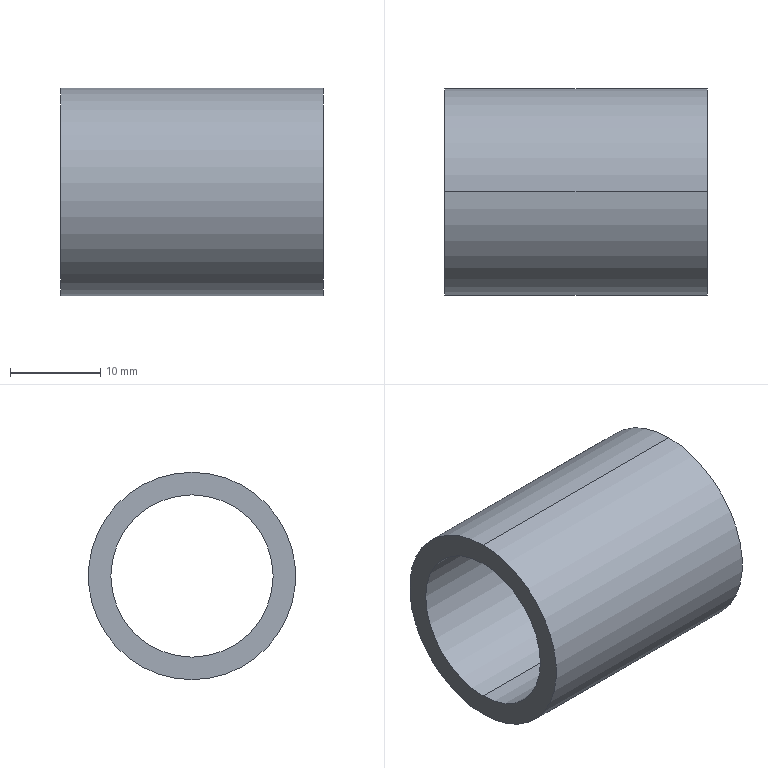Part | STEP file | Completa.sldasm-Part-1_Valor predeterminado | 1 solid | 6 faces | box 29.178 x 23 x 23 mm | volume 4698 mm3 | cylinder 4 | plane 2 | commonest cylinder face diameters 18 x2 23 x2
STEP:
#1=CARTESIAN_POINT('',(0.,0.,0.));
#2=DIRECTION('',(0.,0.,1.));
#3=DIRECTION('',(1.,0.,0.));
#4=AXIS2_PLACEMENT_3D('',#1,#2,#3);
#5=CARTESIAN_POINT('',(-311.426,0.,9.));
#6=VERTEX_POINT('',#5);
#7=CARTESIAN_POINT('',(-340.603,0.,9.));
#8=VERTEX_POINT('',#7);
#9=CARTESIAN_POINT('',(-317.916,0.,9.));
#10=DIRECTION('',(-1.,0.,0.));
#11=VECTOR('',#10,1.);
#12=LINE('',#9,#11);
#13=CARTESIAN_POINT('',(-317.916,0.,0.));
#14=DIRECTION('',(-1.,0.,0.));
#15=DIRECTION('',(0.,0.,1.));
#16=AXIS2_PLACEMENT_3D('',#13,#14,#15);
#17=CYLINDRICAL_SURFACE('',#16,9.);
#18=CARTESIAN_POINT('',(6.283,0.));
#19=DIRECTION('',(0.,1.));
#20=VECTOR('',#19,1.);
#21=LINE('',#18,#20);
#22=(GEOMETRIC_REPRESENTATION_CONTEXT(2)PARAMETRIC_REPRESENTATION_CONTEXT()REPRESENTATION_CONTEXT('',''));
#23=DEFINITIONAL_REPRESENTATION('',(#21),#22);
#24=PCURVE('',#17,#23);
#25=CARTESIAN_POINT('',(-317.916,0.,0.));
#26=DIRECTION('',(-1.,0.,0.));
#27=DIRECTION('',(0.,0.,1.));
#28=AXIS2_PLACEMENT_3D('',#25,#26,#27);
#29=CYLINDRICAL_SURFACE('',#28,9.);
#30=CARTESIAN_POINT('',(0.,0.));
#31=DIRECTION('',(0.,1.));
#32=VECTOR('',#31,1.);
#33=LINE('',#30,#32);
#34=(GEOMETRIC_REPRESENTATION_CONTEXT(2)PARAMETRIC_REPRESENTATION_CONTEXT()REPRESENTATION_CONTEXT('',''));
#35=DEFINITIONAL_REPRESENTATION('',(#33),#34);
#36=PCURVE('',#29,#35);
#37=SURFACE_CURVE('',#12,(#24,#36),.PCURVE_S1.);
#38=EDGE_CURVE('',#6,#8,#37,.T.);
#39=ORIENTED_EDGE('',*,*,#38,.T.);
#40=CARTESIAN_POINT('',(-340.603,0.,-9.));
#41=VERTEX_POINT('',#40);
#42=CARTESIAN_POINT('',(-340.603,0.,0.));
#43=DIRECTION('',(-1.,0.,0.));
#44=DIRECTION('',(0.,0.,-1.));
#45=AXIS2_PLACEMENT_3D('',#42,#43,#44);
#46=CIRCLE('',#45,9.);
#47=CARTESIAN_POINT('',(3.142,22.687));
#48=DIRECTION('',(1.,0.));
#49=VECTOR('',#48,1.);
#50=LINE('',#47,#49);
#51=(GEOMETRIC_REPRESENTATION_CONTEXT(2)PARAMETRIC_REPRESENTATION_CONTEXT()REPRESENTATION_CONTEXT('',''));
#52=DEFINITIONAL_REPRESENTATION('',(#50),#51);
#53=PCURVE('',#17,#52);
#54=CARTESIAN_POINT('',(-340.603,0.,0.));
#55=DIRECTION('',(1.,0.,0.));
#56=DIRECTION('',(0.,0.,-1.));
#57=AXIS2_PLACEMENT_3D('',#54,#55,#56);
#58=PLANE('',#57);
#59=CARTESIAN_POINT('',(9.,0.));
#60=CARTESIAN_POINT('',(9.,-15.588));
#61=CARTESIAN_POINT('',(-4.5,-7.794));
#62=CARTESIAN_POINT('',(-18.,0.));
#63=CARTESIAN_POINT('',(-4.5,7.794));
#64=CARTESIAN_POINT('',(9.,15.588));
#65=CARTESIAN_POINT('',(9.,0.));
#66=(BOUNDED_CURVE()B_SPLINE_CURVE(2,(#59,#60,#61,#62,#63,#64,#65),.UNSPECIFIED.,.T.,.F.)B_SPLINE_CURVE_WITH_KNOTS((1,2,2,2,2,1),(-2.094,0.,2.094,4.189,6.283,8.378),.UNSPECIFIED.)CURVE()GEOMETRIC_REPRESENTATION_ITEM()RATIONAL_B_SPLINE_CURVE((1.,0.5,1.,0.5,1.,0.5,1.))REPRESENTATION_ITEM(''));
#67=(GEOMETRIC_REPRESENTATION_CONTEXT(2)PARAMETRIC_REPRESENTATION_CONTEXT()REPRESENTATION_CONTEXT('',''));
#68=DEFINITIONAL_REPRESENTATION('',(#66),#67);
#69=PCURVE('',#58,#68);
#70=SURFACE_CURVE('',#46,(#53,#69),.PCURVE_S1.);
#71=EDGE_CURVE('',#41,#8,#70,.T.);
#72=ORIENTED_EDGE('',*,*,#71,.F.);
#73=CARTESIAN_POINT('',(-311.426,0.,-9.));
#74=VERTEX_POINT('',#73);
#75=CARTESIAN_POINT('',(-317.916,0.,-9.));
#76=DIRECTION('',(-1.,0.,0.));
#77=VECTOR('',#76,1.);
#78=LINE('',#75,#77);
#79=CARTESIAN_POINT('',(3.142,0.));
#80=DIRECTION('',(0.,1.));
#81=VECTOR('',#80,1.);
#82=LINE('',#79,#81);
#83=(GEOMETRIC_REPRESENTATION_CONTEXT(2)PARAMETRIC_REPRESENTATION_CONTEXT()REPRESENTATION_CONTEXT('',''));
#84=DEFINITIONAL_REPRESENTATION('',(#82),#83);
#85=PCURVE('',#17,#84);
#86=CARTESIAN_POINT('',(3.142,0.));
#87=DIRECTION('',(0.,1.));
#88=VECTOR('',#87,1.);
#89=LINE('',#86,#88);
#90=(GEOMETRIC_REPRESENTATION_CONTEXT(2)PARAMETRIC_REPRESENTATION_CONTEXT()REPRESENTATION_CONTEXT('',''));
#91=DEFINITIONAL_REPRESENTATION('',(#89),#90);
#92=PCURVE('',#29,#91);
#93=SURFACE_CURVE('',#78,(#85,#92),.PCURVE_S1.);
#94=EDGE_CURVE('',#74,#41,#93,.T.);
#95=ORIENTED_EDGE('',*,*,#94,.F.);
#96=CARTESIAN_POINT('',(-311.426,0.,0.));
#97=DIRECTION('',(1.,0.,0.));
#98=DIRECTION('',(0.,0.,1.));
#99=AXIS2_PLACEMENT_3D('',#96,#97,#98);
#100=CIRCLE('',#99,9.);
#101=CARTESIAN_POINT('',(6.283,-6.49));
#102=DIRECTION('',(-1.,0.));
#103=VECTOR('',#102,1.);
#104=LINE('',#101,#103);
#105=(GEOMETRIC_REPRESENTATION_CONTEXT(2)PARAMETRIC_REPRESENTATION_CONTEXT()REPRESENTATION_CONTEXT('',''));
#106=DEFINITIONAL_REPRESENTATION('',(#104),#105);
#107=PCURVE('',#17,#106);
#108=CARTESIAN_POINT('',(-311.426,0.,0.));
#109=DIRECTION('',(-1.,0.,0.));
#110=DIRECTION('',(0.,0.,1.));
#111=AXIS2_PLACEMENT_3D('',#108,#109,#110);
#112=PLANE('',#111);
#113=CARTESIAN_POINT('',(9.,0.));
#114=CARTESIAN_POINT('',(9.,-15.588));
#115=CARTESIAN_POINT('',(-4.5,-7.794));
#116=CARTESIAN_POINT('',(-18.,0.));
#117=CARTESIAN_POINT('',(-4.5,7.794));
#118=CARTESIAN_POINT('',(9.,15.588));
#119=CARTESIAN_POINT('',(9.,0.));
#120=(BOUNDED_CURVE()B_SPLINE_CURVE(2,(#113,#114,#115,#116,#117,#118,#119),.UNSPECIFIED.,.T.,.F.)B_SPLINE_CURVE_WITH_KNOTS((1,2,2,2,2,1),(-2.094,0.,2.094,4.189,6.283,8.378),.UNSPECIFIED.)CURVE()GEOMETRIC_REPRESENTATION_ITEM()RATIONAL_B_SPLINE_CURVE((1.,0.5,1.,0.5,1.,0.5,1.))REPRESENTATION_ITEM(''));
#121=(GEOMETRIC_REPRESENTATION_CONTEXT(2)PARAMETRIC_REPRESENTATION_CONTEXT()REPRESENTATION_CONTEXT('',''));
#122=DEFINITIONAL_REPRESENTATION('',(#120),#121);
#123=PCURVE('',#112,#122);
#124=SURFACE_CURVE('',#100,(#107,#123),.PCURVE_S1.);
#125=EDGE_CURVE('',#6,#74,#124,.T.);
#126=ORIENTED_EDGE('',*,*,#125,.F.);
#127=EDGE_LOOP('',(#39,#72,#95,#126));
#128=FACE_BOUND('',#127,.F.);
#129=ADVANCED_FACE('',(#128),#17,.F.);
#130=CARTESIAN_POINT('',(-311.426,0.,-11.5));
#131=VERTEX_POINT('',#130);
#132=CARTESIAN_POINT('',(-311.426,0.,11.5));
#133=VERTEX_POINT('',#132);
#134=CARTESIAN_POINT('',(-311.426,0.,0.));
#135=DIRECTION('',(1.,0.,0.));
#136=DIRECTION('',(0.,0.,1.));
#137=AXIS2_PLACEMENT_3D('',#134,#135,#136);
#138=CIRCLE('',#137,11.5);
#139=CARTESIAN_POINT('',(-317.916,0.,0.));
#140=DIRECTION('',(-1.,0.,0.));
#141=DIRECTION('',(0.,0.,1.));
#142=AXIS2_PLACEMENT_3D('',#139,#140,#141);
#143=CYLINDRICAL_SURFACE('',#142,11.5);
#144=CARTESIAN_POINT('',(6.283,-6.49));
#145=DIRECTION('',(-1.,0.));
#146=VECTOR('',#145,1.);
#147=LINE('',#144,#146);
#148=(GEOMETRIC_REPRESENTATION_CONTEXT(2)PARAMETRIC_REPRESENTATION_CONTEXT()REPRESENTATION_CONTEXT('',''));
#149=DEFINITIONAL_REPRESENTATION('',(#147),#148);
#150=PCURVE('',#143,#149);
#151=CARTESIAN_POINT('',(11.5,0.));
#152=CARTESIAN_POINT('',(11.5,-19.919));
#153=CARTESIAN_POINT('',(-5.75,-9.959));
#154=CARTESIAN_POINT('',(-23.,0.));
#155=CARTESIAN_POINT('',(-5.75,9.959));
#156=CARTESIAN_POINT('',(11.5,19.919));
#157=CARTESIAN_POINT('',(11.5,0.));
#158=(BOUNDED_CURVE()B_SPLINE_CURVE(2,(#151,#152,#153,#154,#155,#156,#157),.UNSPECIFIED.,.T.,.F.)B_SPLINE_CURVE_WITH_KNOTS((1,2,2,2,2,1),(-2.094,0.,2.094,4.189,6.283,8.378),.UNSPECIFIED.)CURVE()GEOMETRIC_REPRESENTATION_ITEM()RATIONAL_B_SPLINE_CURVE((1.,0.5,1.,0.5,1.,0.5,1.))REPRESENTATION_ITEM(''));
#159=(GEOMETRIC_REPRESENTATION_CONTEXT(2)PARAMETRIC_REPRESENTATION_CONTEXT()REPRESENTATION_CONTEXT('',''));
#160=DEFINITIONAL_REPRESENTATION('',(#158),#159);
#161=PCURVE('',#112,#160);
#162=SURFACE_CURVE('',#138,(#150,#161),.PCURVE_S1.);
#163=EDGE_CURVE('',#131,#133,#162,.T.);
#164=ORIENTED_EDGE('',*,*,#163,.F.);
#165=CARTESIAN_POINT('',(-340.603,0.,-11.5));
#166=VERTEX_POINT('',#165);
#167=CARTESIAN_POINT('',(-317.916,0.,-11.5));
#168=DIRECTION('',(-1.,0.,0.));
#169=VECTOR('',#168,1.);
#170=LINE('',#167,#169);
#171=CARTESIAN_POINT('',(3.142,0.));
#172=DIRECTION('',(0.,1.));
#173=VECTOR('',#172,1.);
#174=LINE('',#171,#173);
#175=(GEOMETRIC_REPRESENTATION_CONTEXT(2)PARAMETRIC_REPRESENTATION_CONTEXT()REPRESENTATION_CONTEXT('',''));
#176=DEFINITIONAL_REPRESENTATION('',(#174),#175);
#177=PCURVE('',#143,#176);
#178=CARTESIAN_POINT('',(-317.916,0.,0.));
#179=DIRECTION('',(-1.,0.,0.));
#180=DIRECTION('',(0.,0.,1.));
#181=AXIS2_PLACEMENT_3D('',#178,#179,#180);
#182=CYLINDRICAL_SURFACE('',#181,11.5);
#183=CARTESIAN_POINT('',(3.142,0.));
#184=DIRECTION('',(0.,1.));
#185=VECTOR('',#184,1.);
#186=LINE('',#183,#185);
#187=(GEOMETRIC_REPRESENTATION_CONTEXT(2)PARAMETRIC_REPRESENTATION_CONTEXT()REPRESENTATION_CONTEXT('',''));
#188=DEFINITIONAL_REPRESENTATION('',(#186),#187);
#189=PCURVE('',#182,#188);
#190=SURFACE_CURVE('',#170,(#177,#189),.PCURVE_S1.);
#191=EDGE_CURVE('',#131,#166,#190,.T.);
#192=ORIENTED_EDGE('',*,*,#191,.T.);
#193=CARTESIAN_POINT('',(-340.603,0.,11.5));
#194=VERTEX_POINT('',#193);
#195=CARTESIAN_POINT('',(-340.603,0.,0.));
#196=DIRECTION('',(-1.,0.,0.));
#197=DIRECTION('',(0.,0.,-1.));
#198=AXIS2_PLACEMENT_3D('',#195,#196,#197);
#199=CIRCLE('',#198,11.5);
#200=CARTESIAN_POINT('',(-3.142,22.687));
#201=DIRECTION('',(1.,0.));
#202=VECTOR('',#201,1.);
#203=LINE('',#200,#202);
#204=(GEOMETRIC_REPRESENTATION_CONTEXT(2)PARAMETRIC_REPRESENTATION_CONTEXT()REPRESENTATION_CONTEXT('',''));
#205=DEFINITIONAL_REPRESENTATION('',(#203),#204);
#206=PCURVE('',#143,#205);
#207=CARTESIAN_POINT('',(11.5,0.));
#208=CARTESIAN_POINT('',(11.5,-19.919));
#209=CARTESIAN_POINT('',(-5.75,-9.959));
#210=CARTESIAN_POINT('',(-23.,0.));
#211=CARTESIAN_POINT('',(-5.75,9.959));
#212=CARTESIAN_POINT('',(11.5,19.919));
#213=CARTESIAN_POINT('',(11.5,0.));
#214=(BOUNDED_CURVE()B_SPLINE_CURVE(2,(#207,#208,#209,#210,#211,#212,#213),.UNSPECIFIED.,.T.,.F.)B_SPLINE_CURVE_WITH_KNOTS((1,2,2,2,2,1),(-2.094,0.,2.094,4.189,6.283,8.378),.UNSPECIFIED.)CURVE()GEOMETRIC_REPRESENTATION_ITEM()RATIONAL_B_SPLINE_CURVE((1.,0.5,1.,0.5,1.,0.5,1.))REPRESENTATION_ITEM(''));
#215=(GEOMETRIC_REPRESENTATION_CONTEXT(2)PARAMETRIC_REPRESENTATION_CONTEXT()REPRESENTATION_CONTEXT('',''));
#216=DEFINITIONAL_REPRESENTATION('',(#214),#215);
#217=PCURVE('',#58,#216);
#218=SURFACE_CURVE('',#199,(#206,#217),.PCURVE_S1.);
#219=EDGE_CURVE('',#194,#166,#218,.T.);
#220=ORIENTED_EDGE('',*,*,#219,.F.);
#221=CARTESIAN_POINT('',(-317.916,0.,11.5));
#222=DIRECTION('',(-1.,0.,0.));
#223=VECTOR('',#222,1.);
#224=LINE('',#221,#223);
#225=CARTESIAN_POINT('',(0.,0.));
#226=DIRECTION('',(0.,1.));
#227=VECTOR('',#226,1.);
#228=LINE('',#225,#227);
#229=(GEOMETRIC_REPRESENTATION_CONTEXT(2)PARAMETRIC_REPRESENTATION_CONTEXT()REPRESENTATION_CONTEXT('',''));
#230=DEFINITIONAL_REPRESENTATION('',(#228),#229);
#231=PCURVE('',#143,#230);
#232=CARTESIAN_POINT('',(6.283,0.));
#233=DIRECTION('',(0.,1.));
#234=VECTOR('',#233,1.);
#235=LINE('',#232,#234);
#236=(GEOMETRIC_REPRESENTATION_CONTEXT(2)PARAMETRIC_REPRESENTATION_CONTEXT()REPRESENTATION_CONTEXT('',''));
#237=DEFINITIONAL_REPRESENTATION('',(#235),#236);
#238=PCURVE('',#182,#237);
#239=SURFACE_CURVE('',#224,(#231,#238),.PCURVE_S1.);
#240=EDGE_CURVE('',#133,#194,#239,.T.);
#241=ORIENTED_EDGE('',*,*,#240,.F.);
#242=EDGE_LOOP('',(#164,#192,#220,#241));
#243=FACE_BOUND('',#242,.T.);
#244=ADVANCED_FACE('',(#243),#143,.T.);
#245=ORIENTED_EDGE('',*,*,#191,.F.);
#246=CARTESIAN_POINT('',(-311.426,0.,0.));
#247=DIRECTION('',(1.,0.,0.));
#248=DIRECTION('',(0.,0.,1.));
#249=AXIS2_PLACEMENT_3D('',#246,#247,#248);
#250=CIRCLE('',#249,11.5);
#251=CARTESIAN_POINT('',(6.283,-6.49));
#252=DIRECTION('',(-1.,0.));
#253=VECTOR('',#252,1.);
#254=LINE('',#251,#253);
#255=(GEOMETRIC_REPRESENTATION_CONTEXT(2)PARAMETRIC_REPRESENTATION_CONTEXT()REPRESENTATION_CONTEXT('',''));
#256=DEFINITIONAL_REPRESENTATION('',(#254),#255);
#257=PCURVE('',#182,#256);
#258=CARTESIAN_POINT('',(11.5,0.));
#259=CARTESIAN_POINT('',(11.5,-19.919));
#260=CARTESIAN_POINT('',(-5.75,-9.959));
#261=CARTESIAN_POINT('',(-23.,0.));
#262=CARTESIAN_POINT('',(-5.75,9.959));
#263=CARTESIAN_POINT('',(11.5,19.919));
#264=CARTESIAN_POINT('',(11.5,0.));
#265=(BOUNDED_CURVE()B_SPLINE_CURVE(2,(#258,#259,#260,#261,#262,#263,#264),.UNSPECIFIED.,.T.,.F.)B_SPLINE_CURVE_WITH_KNOTS((1,2,2,2,2,1),(-2.094,0.,2.094,4.189,6.283,8.378),.UNSPECIFIED.)CURVE()GEOMETRIC_REPRESENTATION_ITEM()RATIONAL_B_SPLINE_CURVE((1.,0.5,1.,0.5,1.,0.5,1.))REPRESENTATION_ITEM(''));
#266=(GEOMETRIC_REPRESENTATION_CONTEXT(2)PARAMETRIC_REPRESENTATION_CONTEXT()REPRESENTATION_CONTEXT('',''));
#267=DEFINITIONAL_REPRESENTATION('',(#265),#266);
#268=PCURVE('',#112,#267);
#269=SURFACE_CURVE('',#250,(#257,#268),.PCURVE_S1.);
#270=EDGE_CURVE('',#133,#131,#269,.T.);
#271=ORIENTED_EDGE('',*,*,#270,.F.);
#272=ORIENTED_EDGE('',*,*,#240,.T.);
#273=CARTESIAN_POINT('',(-340.603,0.,0.));
#274=DIRECTION('',(-1.,0.,0.));
#275=DIRECTION('',(0.,0.,-1.));
#276=AXIS2_PLACEMENT_3D('',#273,#274,#275);
#277=CIRCLE('',#276,11.5);
#278=CARTESIAN_POINT('',(3.142,22.687));
#279=DIRECTION('',(1.,0.));
#280=VECTOR('',#279,1.);
#281=LINE('',#278,#280);
#282=(GEOMETRIC_REPRESENTATION_CONTEXT(2)PARAMETRIC_REPRESENTATION_CONTEXT()REPRESENTATION_CONTEXT('',''));
#283=DEFINITIONAL_REPRESENTATION('',(#281),#282);
#284=PCURVE('',#182,#283);
#285=CARTESIAN_POINT('',(11.5,0.));
#286=CARTESIAN_POINT('',(11.5,-19.919));
#287=CARTESIAN_POINT('',(-5.75,-9.959));
#288=CARTESIAN_POINT('',(-23.,0.));
#289=CARTESIAN_POINT('',(-5.75,9.959));
#290=CARTESIAN_POINT('',(11.5,19.919));
#291=CARTESIAN_POINT('',(11.5,0.));
#292=(BOUNDED_CURVE()B_SPLINE_CURVE(2,(#285,#286,#287,#288,#289,#290,#291),.UNSPECIFIED.,.T.,.F.)B_SPLINE_CURVE_WITH_KNOTS((1,2,2,2,2,1),(-2.094,0.,2.094,4.189,6.283,8.378),.UNSPECIFIED.)CURVE()GEOMETRIC_REPRESENTATION_ITEM()RATIONAL_B_SPLINE_CURVE((1.,0.5,1.,0.5,1.,0.5,1.))REPRESENTATION_ITEM(''));
#293=(GEOMETRIC_REPRESENTATION_CONTEXT(2)PARAMETRIC_REPRESENTATION_CONTEXT()REPRESENTATION_CONTEXT('',''));
#294=DEFINITIONAL_REPRESENTATION('',(#292),#293);
#295=PCURVE('',#58,#294);
#296=SURFACE_CURVE('',#277,(#284,#295),.PCURVE_S1.);
#297=EDGE_CURVE('',#166,#194,#296,.T.);
#298=ORIENTED_EDGE('',*,*,#297,.F.);
#299=EDGE_LOOP('',(#245,#271,#272,#298));
#300=FACE_BOUND('',#299,.T.);
#301=ADVANCED_FACE('',(#300),#182,.T.);
#302=CARTESIAN_POINT('',(-340.603,0.,0.));
#303=DIRECTION('',(-1.,0.,0.));
#304=DIRECTION('',(0.,0.,-1.));
#305=AXIS2_PLACEMENT_3D('',#302,#303,#304);
#306=CIRCLE('',#305,9.);
#307=CARTESIAN_POINT('',(-3.142,22.687));
#308=DIRECTION('',(1.,0.));
#309=VECTOR('',#308,1.);
#310=LINE('',#307,#309);
#311=(GEOMETRIC_REPRESENTATION_CONTEXT(2)PARAMETRIC_REPRESENTATION_CONTEXT()REPRESENTATION_CONTEXT('',''));
#312=DEFINITIONAL_REPRESENTATION('',(#310),#311);
#313=PCURVE('',#29,#312);
#314=CARTESIAN_POINT('',(9.,0.));
#315=CARTESIAN_POINT('',(9.,-15.588));
#316=CARTESIAN_POINT('',(-4.5,-7.794));
#317=CARTESIAN_POINT('',(-18.,0.));
#318=CARTESIAN_POINT('',(-4.5,7.794));
#319=CARTESIAN_POINT('',(9.,15.588));
#320=CARTESIAN_POINT('',(9.,0.));
#321=(BOUNDED_CURVE()B_SPLINE_CURVE(2,(#314,#315,#316,#317,#318,#319,#320),.UNSPECIFIED.,.T.,.F.)B_SPLINE_CURVE_WITH_KNOTS((1,2,2,2,2,1),(-2.094,0.,2.094,4.189,6.283,8.378),.UNSPECIFIED.)CURVE()GEOMETRIC_REPRESENTATION_ITEM()RATIONAL_B_SPLINE_CURVE((1.,0.5,1.,0.5,1.,0.5,1.))REPRESENTATION_ITEM(''));
#322=(GEOMETRIC_REPRESENTATION_CONTEXT(2)PARAMETRIC_REPRESENTATION_CONTEXT()REPRESENTATION_CONTEXT('',''));
#323=DEFINITIONAL_REPRESENTATION('',(#321),#322);
#324=PCURVE('',#58,#323);
#325=SURFACE_CURVE('',#306,(#313,#324),.PCURVE_S1.);
#326=EDGE_CURVE('',#8,#41,#325,.T.);
#327=ORIENTED_EDGE('',*,*,#326,.F.);
#328=ORIENTED_EDGE('',*,*,#38,.F.);
#329=CARTESIAN_POINT('',(-311.426,0.,0.));
#330=DIRECTION('',(1.,0.,0.));
#331=DIRECTION('',(0.,0.,1.));
#332=AXIS2_PLACEMENT_3D('',#329,#330,#331);
#333=CIRCLE('',#332,9.);
#334=CARTESIAN_POINT('',(6.283,-6.49));
#335=DIRECTION('',(-1.,0.));
#336=VECTOR('',#335,1.);
#337=LINE('',#334,#336);
#338=(GEOMETRIC_REPRESENTATION_CONTEXT(2)PARAMETRIC_REPRESENTATION_CONTEXT()REPRESENTATION_CONTEXT('',''));
#339=DEFINITIONAL_REPRESENTATION('',(#337),#338);
#340=PCURVE('',#29,#339);
#341=CARTESIAN_POINT('',(9.,0.));
#342=CARTESIAN_POINT('',(9.,-15.588));
#343=CARTESIAN_POINT('',(-4.5,-7.794));
#344=CARTESIAN_POINT('',(-18.,0.));
#345=CARTESIAN_POINT('',(-4.5,7.794));
#346=CARTESIAN_POINT('',(9.,15.588));
#347=CARTESIAN_POINT('',(9.,0.));
#348=(BOUNDED_CURVE()B_SPLINE_CURVE(2,(#341,#342,#343,#344,#345,#346,#347),.UNSPECIFIED.,.T.,.F.)B_SPLINE_CURVE_WITH_KNOTS((1,2,2,2,2,1),(-2.094,0.,2.094,4.189,6.283,8.378),.UNSPECIFIED.)CURVE()GEOMETRIC_REPRESENTATION_ITEM()RATIONAL_B_SPLINE_CURVE((1.,0.5,1.,0.5,1.,0.5,1.))REPRESENTATION_ITEM(''));
#349=(GEOMETRIC_REPRESENTATION_CONTEXT(2)PARAMETRIC_REPRESENTATION_CONTEXT()REPRESENTATION_CONTEXT('',''));
#350=DEFINITIONAL_REPRESENTATION('',(#348),#349);
#351=PCURVE('',#112,#350);
#352=SURFACE_CURVE('',#333,(#340,#351),.PCURVE_S1.);
#353=EDGE_CURVE('',#74,#6,#352,.T.);
#354=ORIENTED_EDGE('',*,*,#353,.F.);
#355=ORIENTED_EDGE('',*,*,#94,.T.);
#356=EDGE_LOOP('',(#327,#328,#354,#355));
#357=FACE_BOUND('',#356,.F.);
#358=ADVANCED_FACE('',(#357),#29,.F.);
#359=ORIENTED_EDGE('',*,*,#219,.T.);
#360=ORIENTED_EDGE('',*,*,#297,.T.);
#361=EDGE_LOOP('',(#359,#360));
#362=FACE_BOUND('',#361,.T.);
#363=ORIENTED_EDGE('',*,*,#326,.F.);
#364=ORIENTED_EDGE('',*,*,#71,.F.);
#365=EDGE_LOOP('',(#363,#364));
#366=FACE_BOUND('',#365,.T.);
#367=ADVANCED_FACE('',(#362,#366),#58,.F.);
#368=ORIENTED_EDGE('',*,*,#270,.T.);
#369=ORIENTED_EDGE('',*,*,#163,.T.);
#370=EDGE_LOOP('',(#368,#369));
#371=FACE_BOUND('',#370,.T.);
#372=ORIENTED_EDGE('',*,*,#125,.F.);
#373=ORIENTED_EDGE('',*,*,#353,.F.);
#374=EDGE_LOOP('',(#372,#373));
#375=FACE_BOUND('',#374,.T.);
#376=ADVANCED_FACE('',(#371,#375),#112,.F.);
#377=CLOSED_SHELL('',(#129,#244,#301,#358,#367,#376));
#378=MANIFOLD_SOLID_BREP('',#377);
#379=(LENGTH_UNIT()NAMED_UNIT(*)SI_UNIT(.MILLI.,.METRE.));
#380=UNCERTAINTY_MEASURE_WITH_UNIT(LENGTH_MEASURE(0.0000001),#379,'','');
#381=(NAMED_UNIT(*)PLANE_ANGLE_UNIT()SI_UNIT($,.RADIAN.));
#382=(NAMED_UNIT(*)SI_UNIT($,.STERADIAN.)SOLID_ANGLE_UNIT());
#383=(GEOMETRIC_REPRESENTATION_CONTEXT(3)GLOBAL_UNCERTAINTY_ASSIGNED_CONTEXT((#380))GLOBAL_UNIT_ASSIGNED_CONTEXT((#379,#381,#382))REPRESENTATION_CONTEXT('',''));
#384=ADVANCED_BREP_SHAPE_REPRESENTATION('',(#4,#378),#383);